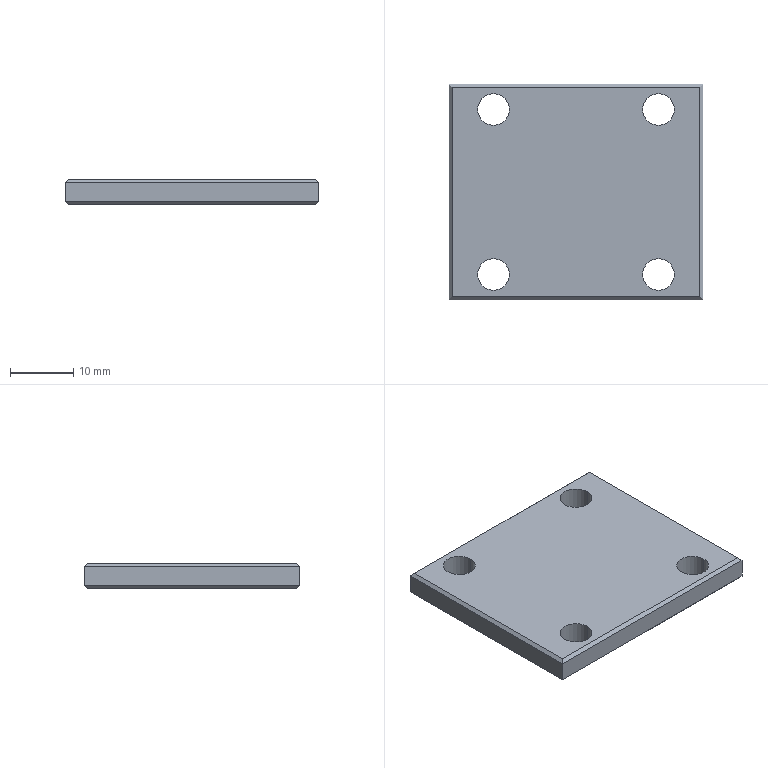Part | NX | 1 solid | 30 faces | box 40 x 34 x 4.05 mm | volume 5145 mm3 | plane 14 | cylinder 8 | cone 8 | commonest cylinder face diameters 5 x8
STEP:
#1=CARTESIAN_POINT('',(0.5,-0.5,3.45));
#2=VERTEX_POINT('',#1);
#3=CARTESIAN_POINT('',(0.5,-33.5,3.45));
#4=VERTEX_POINT('',#3);
#5=CARTESIAN_POINT('',(0.5,0.,3.45));
#6=DIRECTION('',(0.,-1.,0.));
#7=VECTOR('',#6,1000.);
#8=LINE('',#5,#7);
#9=EDGE_CURVE('',#2,#4,#8,.T.);
#10=ORIENTED_EDGE('',*,*,#9,.T.);
#11=CARTESIAN_POINT('',(39.5,-33.5,3.45));
#12=VERTEX_POINT('',#11);
#13=CARTESIAN_POINT('',(0.,-33.5,3.45));
#14=DIRECTION('',(1.,0.,0.));
#15=VECTOR('',#14,1000.);
#16=LINE('',#13,#15);
#17=EDGE_CURVE('',#4,#12,#16,.T.);
#18=ORIENTED_EDGE('',*,*,#17,.T.);
#19=CARTESIAN_POINT('',(39.5,-0.5,3.45));
#20=VERTEX_POINT('',#19);
#21=CARTESIAN_POINT('',(39.5,0.,3.45));
#22=DIRECTION('',(0.,1.,0.));
#23=VECTOR('',#22,1000.);
#24=LINE('',#21,#23);
#25=EDGE_CURVE('',#12,#20,#24,.T.);
#26=ORIENTED_EDGE('',*,*,#25,.T.);
#27=CARTESIAN_POINT('',(0.,-0.5,3.45));
#28=DIRECTION('',(-1.,0.,0.));
#29=VECTOR('',#28,1000.);
#30=LINE('',#27,#29);
#31=EDGE_CURVE('',#20,#2,#30,.T.);
#32=ORIENTED_EDGE('',*,*,#31,.T.);
#33=EDGE_LOOP('',(#10,#18,#26,#32));
#34=FACE_BOUND('',#33,.T.);
#35=CARTESIAN_POINT('',(30.5,-4.,3.45));
#36=VERTEX_POINT('',#35);
#37=CARTESIAN_POINT('',(35.5,-4.,3.45));
#38=VERTEX_POINT('',#37);
#39=CARTESIAN_POINT('',(33.,-4.,3.45));
#40=DIRECTION('',(0.,0.,-1.));
#41=DIRECTION('',(-1.,0.,0.));
#42=AXIS2_PLACEMENT_3D('',#39,#40,#41);
#43=CIRCLE('',#42,2.5);
#44=EDGE_CURVE('',#36,#38,#43,.T.);
#45=ORIENTED_EDGE('',*,*,#44,.T.);
#46=CARTESIAN_POINT('',(33.,-4.,3.45));
#47=DIRECTION('',(0.,0.,-1.));
#48=DIRECTION('',(-1.,0.,0.));
#49=AXIS2_PLACEMENT_3D('',#46,#47,#48);
#50=CIRCLE('',#49,2.5);
#51=EDGE_CURVE('',#38,#36,#50,.T.);
#52=ORIENTED_EDGE('',*,*,#51,.T.);
#53=EDGE_LOOP('',(#45,#52));
#54=FACE_BOUND('',#53,.T.);
#55=CARTESIAN_POINT('',(35.5,-30.,3.45));
#56=VERTEX_POINT('',#55);
#57=CARTESIAN_POINT('',(30.5,-30.,3.45));
#58=VERTEX_POINT('',#57);
#59=CARTESIAN_POINT('',(33.,-30.,3.45));
#60=DIRECTION('',(0.,0.,-1.));
#61=DIRECTION('',(-1.,0.,0.));
#62=AXIS2_PLACEMENT_3D('',#59,#60,#61);
#63=CIRCLE('',#62,2.5);
#64=EDGE_CURVE('',#56,#58,#63,.T.);
#65=ORIENTED_EDGE('',*,*,#64,.T.);
#66=CARTESIAN_POINT('',(33.,-30.,3.45));
#67=DIRECTION('',(0.,0.,-1.));
#68=DIRECTION('',(-1.,0.,0.));
#69=AXIS2_PLACEMENT_3D('',#66,#67,#68);
#70=CIRCLE('',#69,2.5);
#71=EDGE_CURVE('',#58,#56,#70,.T.);
#72=ORIENTED_EDGE('',*,*,#71,.T.);
#73=EDGE_LOOP('',(#65,#72));
#74=FACE_BOUND('',#73,.T.);
#75=CARTESIAN_POINT('',(4.5,-4.,3.45));
#76=VERTEX_POINT('',#75);
#77=CARTESIAN_POINT('',(9.5,-4.,3.45));
#78=VERTEX_POINT('',#77);
#79=CARTESIAN_POINT('',(7.,-4.,3.45));
#80=DIRECTION('',(0.,0.,-1.));
#81=DIRECTION('',(-1.,0.,0.));
#82=AXIS2_PLACEMENT_3D('',#79,#80,#81);
#83=CIRCLE('',#82,2.5);
#84=EDGE_CURVE('',#76,#78,#83,.T.);
#85=ORIENTED_EDGE('',*,*,#84,.T.);
#86=CARTESIAN_POINT('',(7.,-4.,3.45));
#87=DIRECTION('',(0.,0.,-1.));
#88=DIRECTION('',(-1.,0.,0.));
#89=AXIS2_PLACEMENT_3D('',#86,#87,#88);
#90=CIRCLE('',#89,2.5);
#91=EDGE_CURVE('',#78,#76,#90,.T.);
#92=ORIENTED_EDGE('',*,*,#91,.T.);
#93=EDGE_LOOP('',(#85,#92));
#94=FACE_BOUND('',#93,.T.);
#95=CARTESIAN_POINT('',(4.5,-30.,3.45));
#96=VERTEX_POINT('',#95);
#97=CARTESIAN_POINT('',(9.5,-30.,3.45));
#98=VERTEX_POINT('',#97);
#99=CARTESIAN_POINT('',(7.,-30.,3.45));
#100=DIRECTION('',(0.,0.,-1.));
#101=DIRECTION('',(-1.,0.,0.));
#102=AXIS2_PLACEMENT_3D('',#99,#100,#101);
#103=CIRCLE('',#102,2.5);
#104=EDGE_CURVE('',#96,#98,#103,.T.);
#105=ORIENTED_EDGE('',*,*,#104,.T.);
#106=CARTESIAN_POINT('',(7.,-30.,3.45));
#107=DIRECTION('',(0.,0.,-1.));
#108=DIRECTION('',(-1.,0.,0.));
#109=AXIS2_PLACEMENT_3D('',#106,#107,#108);
#110=CIRCLE('',#109,2.5);
#111=EDGE_CURVE('',#98,#96,#110,.T.);
#112=ORIENTED_EDGE('',*,*,#111,.T.);
#113=EDGE_LOOP('',(#105,#112));
#114=FACE_BOUND('',#113,.T.);
#115=CARTESIAN_POINT('',(40.,62.,3.45));
#116=DIRECTION('',(0.,0.,-1.));
#117=DIRECTION('',(0.,-1.,0.));
#118=AXIS2_PLACEMENT_3D('',#115,#116,#117);
#119=PLANE('',#118);
#120=ADVANCED_FACE('',(#34,#54,#74,#94,#114),#119,.F.);
#121=CARTESIAN_POINT('',(0.,-34.,2.95));
#122=VERTEX_POINT('',#121);
#123=CARTESIAN_POINT('',(40.,-34.,2.95));
#124=VERTEX_POINT('',#123);
#125=CARTESIAN_POINT('',(0.,-34.,2.95));
#126=DIRECTION('',(1.,0.,0.));
#127=VECTOR('',#126,1000.);
#128=LINE('',#125,#127);
#129=EDGE_CURVE('',#122,#124,#128,.T.);
#130=ORIENTED_EDGE('',*,*,#129,.F.);
#131=CARTESIAN_POINT('',(0.,-34.,-0.1));
#132=VERTEX_POINT('',#131);
#133=CARTESIAN_POINT('',(0.,-34.,0.));
#134=DIRECTION('',(0.,0.,-1.));
#135=VECTOR('',#134,1000.);
#136=LINE('',#133,#135);
#137=EDGE_CURVE('',#122,#132,#136,.T.);
#138=ORIENTED_EDGE('',*,*,#137,.T.);
#139=CARTESIAN_POINT('',(40.,-34.,-0.1));
#140=VERTEX_POINT('',#139);
#141=CARTESIAN_POINT('',(0.,-34.,-0.1));
#142=DIRECTION('',(-1.,0.,0.));
#143=VECTOR('',#142,1000.);
#144=LINE('',#141,#143);
#145=EDGE_CURVE('',#140,#132,#144,.T.);
#146=ORIENTED_EDGE('',*,*,#145,.F.);
#147=CARTESIAN_POINT('',(40.,-34.,0.));
#148=DIRECTION('',(0.,0.,1.));
#149=VECTOR('',#148,1000.);
#150=LINE('',#147,#149);
#151=EDGE_CURVE('',#140,#124,#150,.T.);
#152=ORIENTED_EDGE('',*,*,#151,.T.);
#153=EDGE_LOOP('',(#130,#138,#146,#152));
#154=FACE_BOUND('',#153,.T.);
#155=CARTESIAN_POINT('',(0.,-34.,0.));
#156=DIRECTION('',(0.,-1.,0.));
#157=DIRECTION('',(0.,0.,-1.));
#158=AXIS2_PLACEMENT_3D('',#155,#156,#157);
#159=PLANE('',#158);
#160=ADVANCED_FACE('',(#154),#159,.T.);
#161=ORIENTED_EDGE('',*,*,#44,.F.);
#162=CARTESIAN_POINT('',(30.5,-4.,-0.1));
#163=VERTEX_POINT('',#162);
#164=CARTESIAN_POINT('',(30.5,-4.,10.5));
#165=DIRECTION('',(0.,0.,-1.));
#166=VECTOR('',#165,1000.);
#167=LINE('',#164,#166);
#168=EDGE_CURVE('',#163,#36,#167,.F.);
#169=ORIENTED_EDGE('',*,*,#168,.F.);
#170=CARTESIAN_POINT('',(35.5,-4.,-0.1));
#171=VERTEX_POINT('',#170);
#172=CARTESIAN_POINT('',(33.,-4.,-0.1));
#173=DIRECTION('',(0.,0.,-1.));
#174=DIRECTION('',(-1.,0.,0.));
#175=AXIS2_PLACEMENT_3D('',#172,#173,#174);
#176=CIRCLE('',#175,2.5);
#177=EDGE_CURVE('',#163,#171,#176,.T.);
#178=ORIENTED_EDGE('',*,*,#177,.T.);
#179=CARTESIAN_POINT('',(35.5,-4.,10.5));
#180=DIRECTION('',(0.,0.,-1.));
#181=VECTOR('',#180,1000.);
#182=LINE('',#179,#181);
#183=EDGE_CURVE('',#171,#38,#182,.F.);
#184=ORIENTED_EDGE('',*,*,#183,.T.);
#185=EDGE_LOOP('',(#161,#169,#178,#184));
#186=FACE_BOUND('',#185,.T.);
#187=CARTESIAN_POINT('',(33.,-4.,10.5));
#188=DIRECTION('',(0.,0.,-1.));
#189=DIRECTION('',(-1.,0.,0.));
#190=AXIS2_PLACEMENT_3D('',#187,#188,#189);
#191=CYLINDRICAL_SURFACE('',#190,2.5);
#192=ADVANCED_FACE('',(#186),#191,.F.);
#193=ORIENTED_EDGE('',*,*,#104,.F.);
#194=CARTESIAN_POINT('',(4.5,-30.,-0.1));
#195=VERTEX_POINT('',#194);
#196=CARTESIAN_POINT('',(4.5,-30.,10.5));
#197=DIRECTION('',(0.,0.,-1.));
#198=VECTOR('',#197,1000.);
#199=LINE('',#196,#198);
#200=EDGE_CURVE('',#195,#96,#199,.F.);
#201=ORIENTED_EDGE('',*,*,#200,.F.);
#202=CARTESIAN_POINT('',(9.5,-30.,-0.1));
#203=VERTEX_POINT('',#202);
#204=CARTESIAN_POINT('',(7.,-30.,-0.1));
#205=DIRECTION('',(0.,0.,-1.));
#206=DIRECTION('',(-1.,0.,0.));
#207=AXIS2_PLACEMENT_3D('',#204,#205,#206);
#208=CIRCLE('',#207,2.5);
#209=EDGE_CURVE('',#195,#203,#208,.T.);
#210=ORIENTED_EDGE('',*,*,#209,.T.);
#211=CARTESIAN_POINT('',(9.5,-30.,10.5));
#212=DIRECTION('',(0.,0.,-1.));
#213=VECTOR('',#212,1000.);
#214=LINE('',#211,#213);
#215=EDGE_CURVE('',#203,#98,#214,.F.);
#216=ORIENTED_EDGE('',*,*,#215,.T.);
#217=EDGE_LOOP('',(#193,#201,#210,#216));
#218=FACE_BOUND('',#217,.T.);
#219=CARTESIAN_POINT('',(7.,-30.,10.5));
#220=DIRECTION('',(0.,0.,-1.));
#221=DIRECTION('',(-1.,0.,0.));
#222=AXIS2_PLACEMENT_3D('',#219,#220,#221);
#223=CYLINDRICAL_SURFACE('',#222,2.5);
#224=ADVANCED_FACE('',(#218),#223,.F.);
#225=CARTESIAN_POINT('',(9.5,-4.,-0.1));
#226=VERTEX_POINT('',#225);
#227=CARTESIAN_POINT('',(4.5,-4.,-0.1));
#228=VERTEX_POINT('',#227);
#229=CARTESIAN_POINT('',(7.,-4.,-0.1));
#230=DIRECTION('',(0.,0.,-1.));
#231=DIRECTION('',(-1.,0.,0.));
#232=AXIS2_PLACEMENT_3D('',#229,#230,#231);
#233=CIRCLE('',#232,2.5);
#234=EDGE_CURVE('',#226,#228,#233,.T.);
#235=ORIENTED_EDGE('',*,*,#234,.T.);
#236=CARTESIAN_POINT('',(4.5,-4.,10.5));
#237=DIRECTION('',(0.,0.,-1.));
#238=VECTOR('',#237,1000.);
#239=LINE('',#236,#238);
#240=EDGE_CURVE('',#228,#76,#239,.F.);
#241=ORIENTED_EDGE('',*,*,#240,.T.);
#242=ORIENTED_EDGE('',*,*,#91,.F.);
#243=CARTESIAN_POINT('',(9.5,-4.,10.5));
#244=DIRECTION('',(0.,0.,-1.));
#245=VECTOR('',#244,1000.);
#246=LINE('',#243,#245);
#247=EDGE_CURVE('',#226,#78,#246,.F.);
#248=ORIENTED_EDGE('',*,*,#247,.F.);
#249=EDGE_LOOP('',(#235,#241,#242,#248));
#250=FACE_BOUND('',#249,.T.);
#251=CARTESIAN_POINT('',(7.,-4.,10.5));
#252=DIRECTION('',(0.,0.,-1.));
#253=DIRECTION('',(-1.,0.,0.));
#254=AXIS2_PLACEMENT_3D('',#251,#252,#253);
#255=CYLINDRICAL_SURFACE('',#254,2.5);
#256=ADVANCED_FACE('',(#250),#255,.F.);
#257=CARTESIAN_POINT('',(0.,0.,2.95));
#258=VERTEX_POINT('',#257);
#259=CARTESIAN_POINT('',(0.,0.,2.95));
#260=DIRECTION('',(0.,-1.,0.));
#261=VECTOR('',#260,1000.);
#262=LINE('',#259,#261);
#263=EDGE_CURVE('',#258,#122,#262,.T.);
#264=ORIENTED_EDGE('',*,*,#263,.F.);
#265=CARTESIAN_POINT('',(0.,0.,-0.1));
#266=VERTEX_POINT('',#265);
#267=CARTESIAN_POINT('',(0.,0.,0.));
#268=DIRECTION('',(0.,0.,1.));
#269=VECTOR('',#268,1000.);
#270=LINE('',#267,#269);
#271=EDGE_CURVE('',#266,#258,#270,.T.);
#272=ORIENTED_EDGE('',*,*,#271,.F.);
#273=CARTESIAN_POINT('',(0.,0.,-0.1));
#274=DIRECTION('',(0.,-1.,0.));
#275=VECTOR('',#274,1000.);
#276=LINE('',#273,#275);
#277=EDGE_CURVE('',#266,#132,#276,.T.);
#278=ORIENTED_EDGE('',*,*,#277,.T.);
#279=ORIENTED_EDGE('',*,*,#137,.F.);
#280=EDGE_LOOP('',(#264,#272,#278,#279));
#281=FACE_BOUND('',#280,.T.);
#282=CARTESIAN_POINT('',(0.,0.,0.));
#283=DIRECTION('',(-1.,0.,0.));
#284=DIRECTION('',(0.,0.,1.));
#285=AXIS2_PLACEMENT_3D('',#282,#283,#284);
#286=PLANE('',#285);
#287=ADVANCED_FACE('',(#281),#286,.T.);
#288=ORIENTED_EDGE('',*,*,#64,.F.);
#289=CARTESIAN_POINT('',(35.5,-30.,-0.1));
#290=VERTEX_POINT('',#289);
#291=CARTESIAN_POINT('',(35.5,-30.,10.5));
#292=DIRECTION('',(0.,0.,-1.));
#293=VECTOR('',#292,1000.);
#294=LINE('',#291,#293);
#295=EDGE_CURVE('',#290,#56,#294,.F.);
#296=ORIENTED_EDGE('',*,*,#295,.F.);
#297=CARTESIAN_POINT('',(30.5,-30.,-0.1));
#298=VERTEX_POINT('',#297);
#299=CARTESIAN_POINT('',(33.,-30.,-0.1));
#300=DIRECTION('',(0.,0.,-1.));
#301=DIRECTION('',(-1.,0.,0.));
#302=AXIS2_PLACEMENT_3D('',#299,#300,#301);
#303=CIRCLE('',#302,2.5);
#304=EDGE_CURVE('',#290,#298,#303,.T.);
#305=ORIENTED_EDGE('',*,*,#304,.T.);
#306=CARTESIAN_POINT('',(30.5,-30.,10.5));
#307=DIRECTION('',(0.,0.,-1.));
#308=VECTOR('',#307,1000.);
#309=LINE('',#306,#308);
#310=EDGE_CURVE('',#298,#58,#309,.F.);
#311=ORIENTED_EDGE('',*,*,#310,.T.);
#312=EDGE_LOOP('',(#288,#296,#305,#311));
#313=FACE_BOUND('',#312,.T.);
#314=CARTESIAN_POINT('',(33.,-30.,10.5));
#315=DIRECTION('',(0.,0.,-1.));
#316=DIRECTION('',(-1.,0.,0.));
#317=AXIS2_PLACEMENT_3D('',#314,#315,#316);
#318=CYLINDRICAL_SURFACE('',#317,2.5);
#319=ADVANCED_FACE('',(#313),#318,.F.);
#320=CARTESIAN_POINT('',(33.,-4.,-0.1));
#321=DIRECTION('',(0.,0.,-1.));
#322=DIRECTION('',(-1.,0.,0.));
#323=AXIS2_PLACEMENT_3D('',#320,#321,#322);
#324=CIRCLE('',#323,2.5);
#325=EDGE_CURVE('',#171,#163,#324,.T.);
#326=ORIENTED_EDGE('',*,*,#325,.F.);
#327=CARTESIAN_POINT('',(36.,-4.,-0.6));
#328=VERTEX_POINT('',#327);
#329=CARTESIAN_POINT('',(36.,-4.,-0.6));
#330=DIRECTION('',(0.7071,0.,-0.7071));
#331=VECTOR('',#330,1000.);
#332=LINE('',#329,#331);
#333=EDGE_CURVE('',#171,#328,#332,.T.);
#334=ORIENTED_EDGE('',*,*,#333,.T.);
#335=CARTESIAN_POINT('',(30.,-4.,-0.6));
#336=VERTEX_POINT('',#335);
#337=CARTESIAN_POINT('',(33.,-4.,-0.6));
#338=DIRECTION('',(0.,0.,-1.));
#339=DIRECTION('',(-1.,0.,0.));
#340=AXIS2_PLACEMENT_3D('',#337,#338,#339);
#341=CIRCLE('',#340,3.);
#342=EDGE_CURVE('',#328,#336,#341,.T.);
#343=ORIENTED_EDGE('',*,*,#342,.T.);
#344=CARTESIAN_POINT('',(30.,-4.,-0.6));
#345=DIRECTION('',(-0.7071,0.,-0.7071));
#346=VECTOR('',#345,1000.);
#347=LINE('',#344,#346);
#348=EDGE_CURVE('',#163,#336,#347,.T.);
#349=ORIENTED_EDGE('',*,*,#348,.F.);
#350=EDGE_LOOP('',(#326,#334,#343,#349));
#351=FACE_BOUND('',#350,.T.);
#352=CARTESIAN_POINT('',(33.,-4.,-0.6));
#353=DIRECTION('',(0.,0.,-1.));
#354=DIRECTION('',(-1.,0.,0.));
#355=AXIS2_PLACEMENT_3D('',#352,#353,#354);
#356=CONICAL_SURFACE('',#355,3.,0.7854);
#357=ADVANCED_FACE('',(#351),#356,.F.);
#358=CARTESIAN_POINT('',(40.,0.,2.95));
#359=VERTEX_POINT('',#358);
#360=CARTESIAN_POINT('',(0.,0.,2.95));
#361=DIRECTION('',(-1.,0.,0.));
#362=VECTOR('',#361,1000.);
#363=LINE('',#360,#362);
#364=EDGE_CURVE('',#359,#258,#363,.T.);
#365=ORIENTED_EDGE('',*,*,#364,.F.);
#366=CARTESIAN_POINT('',(40.,0.,-0.1));
#367=VERTEX_POINT('',#366);
#368=CARTESIAN_POINT('',(40.,0.,0.));
#369=DIRECTION('',(0.,0.,-1.));
#370=VECTOR('',#369,1000.);
#371=LINE('',#368,#370);
#372=EDGE_CURVE('',#359,#367,#371,.T.);
#373=ORIENTED_EDGE('',*,*,#372,.T.);
#374=CARTESIAN_POINT('',(0.,0.,-0.1));
#375=DIRECTION('',(1.,0.,0.));
#376=VECTOR('',#375,1000.);
#377=LINE('',#374,#376);
#378=EDGE_CURVE('',#266,#367,#377,.T.);
#379=ORIENTED_EDGE('',*,*,#378,.F.);
#380=ORIENTED_EDGE('',*,*,#271,.T.);
#381=EDGE_LOOP('',(#365,#373,#379,#380));
#382=FACE_BOUND('',#381,.T.);
#383=CARTESIAN_POINT('',(40.,0.,0.));
#384=DIRECTION('',(0.,1.,0.));
#385=DIRECTION('',(1.,0.,0.));
#386=AXIS2_PLACEMENT_3D('',#383,#384,#385);
#387=PLANE('',#386);
#388=ADVANCED_FACE('',(#382),#387,.T.);
#389=CARTESIAN_POINT('',(40.,0.,2.95));
#390=DIRECTION('',(0.,1.,0.));
#391=VECTOR('',#390,1000.);
#392=LINE('',#389,#391);
#393=EDGE_CURVE('',#124,#359,#392,.T.);
#394=ORIENTED_EDGE('',*,*,#393,.F.);
#395=ORIENTED_EDGE('',*,*,#151,.F.);
#396=CARTESIAN_POINT('',(40.,0.,-0.1));
#397=DIRECTION('',(0.,1.,0.));
#398=VECTOR('',#397,1000.);
#399=LINE('',#396,#398);
#400=EDGE_CURVE('',#140,#367,#399,.T.);
#401=ORIENTED_EDGE('',*,*,#400,.T.);
#402=ORIENTED_EDGE('',*,*,#372,.F.);
#403=EDGE_LOOP('',(#394,#395,#401,#402));
#404=FACE_BOUND('',#403,.T.);
#405=CARTESIAN_POINT('',(40.,-34.,0.));
#406=DIRECTION('',(1.,0.,0.));
#407=DIRECTION('',(0.,1.,0.));
#408=AXIS2_PLACEMENT_3D('',#405,#406,#407);
#409=PLANE('',#408);
#410=ADVANCED_FACE('',(#404),#409,.T.);
#411=CARTESIAN_POINT('',(39.5,-0.5,-0.6));
#412=VERTEX_POINT('',#411);
#413=CARTESIAN_POINT('',(39.5,-33.5,-0.6));
#414=VERTEX_POINT('',#413);
#415=CARTESIAN_POINT('',(39.5,0.,-0.6));
#416=DIRECTION('',(0.,-1.,0.));
#417=VECTOR('',#416,1000.);
#418=LINE('',#415,#417);
#419=EDGE_CURVE('',#412,#414,#418,.T.);
#420=ORIENTED_EDGE('',*,*,#419,.F.);
#421=CARTESIAN_POINT('',(40.1,0.1,0.));
#422=DIRECTION('',(0.5774,0.5774,0.5774));
#423=VECTOR('',#422,1000.);
#424=LINE('',#421,#423);
#425=EDGE_CURVE('',#412,#367,#424,.T.);
#426=ORIENTED_EDGE('',*,*,#425,.T.);
#427=ORIENTED_EDGE('',*,*,#400,.F.);
#428=CARTESIAN_POINT('',(40.1,-34.1,0.));
#429=DIRECTION('',(-0.5774,0.5774,-0.5774));
#430=VECTOR('',#429,1000.);
#431=LINE('',#428,#430);
#432=EDGE_CURVE('',#140,#414,#431,.T.);
#433=ORIENTED_EDGE('',*,*,#432,.T.);
#434=EDGE_LOOP('',(#420,#426,#427,#433));
#435=FACE_BOUND('',#434,.T.);
#436=CARTESIAN_POINT('',(39.75,-17.,-0.35));
#437=DIRECTION('',(-0.7071,0.,0.7071));
#438=DIRECTION('',(0.,1.,0.));
#439=AXIS2_PLACEMENT_3D('',#436,#437,#438);
#440=PLANE('',#439);
#441=ADVANCED_FACE('',(#435),#440,.F.);
#442=CARTESIAN_POINT('',(0.5,-33.5,-0.6));
#443=VERTEX_POINT('',#442);
#444=CARTESIAN_POINT('',(0.,-33.5,-0.6));
#445=DIRECTION('',(-1.,0.,0.));
#446=VECTOR('',#445,1000.);
#447=LINE('',#444,#446);
#448=EDGE_CURVE('',#414,#443,#447,.T.);
#449=ORIENTED_EDGE('',*,*,#448,.F.);
#450=ORIENTED_EDGE('',*,*,#432,.F.);
#451=ORIENTED_EDGE('',*,*,#145,.T.);
#452=CARTESIAN_POINT('',(-0.1,-34.1,0.));
#453=DIRECTION('',(-0.5774,-0.5774,0.5774));
#454=VECTOR('',#453,1000.);
#455=LINE('',#452,#454);
#456=EDGE_CURVE('',#443,#132,#455,.T.);
#457=ORIENTED_EDGE('',*,*,#456,.F.);
#458=EDGE_LOOP('',(#449,#450,#451,#457));
#459=FACE_BOUND('',#458,.T.);
#460=CARTESIAN_POINT('',(20.,-33.75,-0.35));
#461=DIRECTION('',(0.,0.7071,0.7071));
#462=DIRECTION('',(1.,0.,0.));
#463=AXIS2_PLACEMENT_3D('',#460,#461,#462);
#464=PLANE('',#463);
#465=ADVANCED_FACE('',(#459),#464,.F.);
#466=CARTESIAN_POINT('',(0.5,-0.5,-0.6));
#467=VERTEX_POINT('',#466);
#468=CARTESIAN_POINT('',(0.5,0.,-0.6));
#469=DIRECTION('',(0.,1.,0.));
#470=VECTOR('',#469,1000.);
#471=LINE('',#468,#470);
#472=EDGE_CURVE('',#443,#467,#471,.T.);
#473=ORIENTED_EDGE('',*,*,#472,.F.);
#474=ORIENTED_EDGE('',*,*,#456,.T.);
#475=ORIENTED_EDGE('',*,*,#277,.F.);
#476=CARTESIAN_POINT('',(-0.1,0.1,0.));
#477=DIRECTION('',(0.5774,-0.5774,-0.5774));
#478=VECTOR('',#477,1000.);
#479=LINE('',#476,#478);
#480=EDGE_CURVE('',#266,#467,#479,.T.);
#481=ORIENTED_EDGE('',*,*,#480,.T.);
#482=EDGE_LOOP('',(#473,#474,#475,#481));
#483=FACE_BOUND('',#482,.T.);
#484=CARTESIAN_POINT('',(0.25,-17.,-0.35));
#485=DIRECTION('',(0.7071,0.,0.7071));
#486=DIRECTION('',(0.,-1.,0.));
#487=AXIS2_PLACEMENT_3D('',#484,#485,#486);
#488=PLANE('',#487);
#489=ADVANCED_FACE('',(#483),#488,.F.);
#490=CARTESIAN_POINT('',(0.,-0.5,-0.6));
#491=DIRECTION('',(1.,0.,0.));
#492=VECTOR('',#491,1000.);
#493=LINE('',#490,#492);
#494=EDGE_CURVE('',#467,#412,#493,.T.);
#495=ORIENTED_EDGE('',*,*,#494,.F.);
#496=ORIENTED_EDGE('',*,*,#480,.F.);
#497=ORIENTED_EDGE('',*,*,#378,.T.);
#498=ORIENTED_EDGE('',*,*,#425,.F.);
#499=EDGE_LOOP('',(#495,#496,#497,#498));
#500=FACE_BOUND('',#499,.T.);
#501=CARTESIAN_POINT('',(20.,-0.25,-0.35));
#502=DIRECTION('',(0.,-0.7071,0.7071));
#503=DIRECTION('',(-1.,0.,0.));
#504=AXIS2_PLACEMENT_3D('',#501,#502,#503);
#505=PLANE('',#504);
#506=ADVANCED_FACE('',(#500),#505,.F.);
#507=CARTESIAN_POINT('',(4.,-30.,-0.6));
#508=VERTEX_POINT('',#507);
#509=CARTESIAN_POINT('',(10.,-30.,-0.6));
#510=VERTEX_POINT('',#509);
#511=CARTESIAN_POINT('',(7.,-30.,-0.6));
#512=DIRECTION('',(0.,0.,-1.));
#513=DIRECTION('',(-1.,0.,0.));
#514=AXIS2_PLACEMENT_3D('',#511,#512,#513);
#515=CIRCLE('',#514,3.);
#516=EDGE_CURVE('',#508,#510,#515,.T.);
#517=ORIENTED_EDGE('',*,*,#516,.T.);
#518=CARTESIAN_POINT('',(10.,-30.,-0.6));
#519=DIRECTION('',(0.7071,0.,-0.7071));
#520=VECTOR('',#519,1000.);
#521=LINE('',#518,#520);
#522=EDGE_CURVE('',#203,#510,#521,.T.);
#523=ORIENTED_EDGE('',*,*,#522,.F.);
#524=ORIENTED_EDGE('',*,*,#209,.F.);
#525=CARTESIAN_POINT('',(4.,-30.,-0.6));
#526=DIRECTION('',(-0.7071,0.,-0.7071));
#527=VECTOR('',#526,1000.);
#528=LINE('',#525,#527);
#529=EDGE_CURVE('',#195,#508,#528,.T.);
#530=ORIENTED_EDGE('',*,*,#529,.T.);
#531=EDGE_LOOP('',(#517,#523,#524,#530));
#532=FACE_BOUND('',#531,.T.);
#533=CARTESIAN_POINT('',(7.,-30.,-0.6));
#534=DIRECTION('',(0.,0.,-1.));
#535=DIRECTION('',(-1.,0.,0.));
#536=AXIS2_PLACEMENT_3D('',#533,#534,#535);
#537=CONICAL_SURFACE('',#536,3.,0.7854);
#538=ADVANCED_FACE('',(#532),#537,.F.);
#539=CARTESIAN_POINT('',(4.,-4.,-0.6));
#540=VERTEX_POINT('',#539);
#541=CARTESIAN_POINT('',(10.,-4.,-0.6));
#542=VERTEX_POINT('',#541);
#543=CARTESIAN_POINT('',(7.,-4.,-0.6));
#544=DIRECTION('',(0.,0.,-1.));
#545=DIRECTION('',(-1.,0.,0.));
#546=AXIS2_PLACEMENT_3D('',#543,#544,#545);
#547=CIRCLE('',#546,3.);
#548=EDGE_CURVE('',#540,#542,#547,.T.);
#549=ORIENTED_EDGE('',*,*,#548,.T.);
#550=CARTESIAN_POINT('',(10.,-4.,-0.6));
#551=DIRECTION('',(0.7071,0.,-0.7071));
#552=VECTOR('',#551,1000.);
#553=LINE('',#550,#552);
#554=EDGE_CURVE('',#226,#542,#553,.T.);
#555=ORIENTED_EDGE('',*,*,#554,.F.);
#556=CARTESIAN_POINT('',(7.,-4.,-0.1));
#557=DIRECTION('',(0.,0.,-1.));
#558=DIRECTION('',(-1.,0.,0.));
#559=AXIS2_PLACEMENT_3D('',#556,#557,#558);
#560=CIRCLE('',#559,2.5);
#561=EDGE_CURVE('',#228,#226,#560,.T.);
#562=ORIENTED_EDGE('',*,*,#561,.F.);
#563=CARTESIAN_POINT('',(4.,-4.,-0.6));
#564=DIRECTION('',(-0.7071,0.,-0.7071));
#565=VECTOR('',#564,1000.);
#566=LINE('',#563,#565);
#567=EDGE_CURVE('',#228,#540,#566,.T.);
#568=ORIENTED_EDGE('',*,*,#567,.T.);
#569=EDGE_LOOP('',(#549,#555,#562,#568));
#570=FACE_BOUND('',#569,.T.);
#571=CARTESIAN_POINT('',(7.,-4.,-0.6));
#572=DIRECTION('',(0.,0.,-1.));
#573=DIRECTION('',(-1.,0.,0.));
#574=AXIS2_PLACEMENT_3D('',#571,#572,#573);
#575=CONICAL_SURFACE('',#574,3.,0.7854);
#576=ADVANCED_FACE('',(#570),#575,.F.);
#577=CARTESIAN_POINT('',(30.,-30.,-0.6));
#578=VERTEX_POINT('',#577);
#579=CARTESIAN_POINT('',(36.,-30.,-0.6));
#580=VERTEX_POINT('',#579);
#581=CARTESIAN_POINT('',(33.,-30.,-0.6));
#582=DIRECTION('',(0.,0.,-1.));
#583=DIRECTION('',(-1.,0.,0.));
#584=AXIS2_PLACEMENT_3D('',#581,#582,#583);
#585=CIRCLE('',#584,3.);
#586=EDGE_CURVE('',#578,#580,#585,.T.);
#587=ORIENTED_EDGE('',*,*,#586,.T.);
#588=CARTESIAN_POINT('',(36.,-30.,-0.6));
#589=DIRECTION('',(0.7071,0.,-0.7071));
#590=VECTOR('',#589,1000.);
#591=LINE('',#588,#590);
#592=EDGE_CURVE('',#290,#580,#591,.T.);
#593=ORIENTED_EDGE('',*,*,#592,.F.);
#594=CARTESIAN_POINT('',(33.,-30.,-0.1));
#595=DIRECTION('',(0.,0.,-1.));
#596=DIRECTION('',(-1.,0.,0.));
#597=AXIS2_PLACEMENT_3D('',#594,#595,#596);
#598=CIRCLE('',#597,2.5);
#599=EDGE_CURVE('',#298,#290,#598,.T.);
#600=ORIENTED_EDGE('',*,*,#599,.F.);
#601=CARTESIAN_POINT('',(30.,-30.,-0.6));
#602=DIRECTION('',(-0.7071,0.,-0.7071));
#603=VECTOR('',#602,1000.);
#604=LINE('',#601,#603);
#605=EDGE_CURVE('',#298,#578,#604,.T.);
#606=ORIENTED_EDGE('',*,*,#605,.T.);
#607=EDGE_LOOP('',(#587,#593,#600,#606));
#608=FACE_BOUND('',#607,.T.);
#609=CARTESIAN_POINT('',(33.,-30.,-0.6));
#610=DIRECTION('',(0.,0.,-1.));
#611=DIRECTION('',(-1.,0.,0.));
#612=AXIS2_PLACEMENT_3D('',#609,#610,#611);
#613=CONICAL_SURFACE('',#612,3.,0.7854);
#614=ADVANCED_FACE('',(#608),#613,.F.);
#615=ORIENTED_EDGE('',*,*,#494,.T.);
#616=ORIENTED_EDGE('',*,*,#419,.T.);
#617=ORIENTED_EDGE('',*,*,#448,.T.);
#618=ORIENTED_EDGE('',*,*,#472,.T.);
#619=EDGE_LOOP('',(#615,#616,#617,#618));
#620=FACE_BOUND('',#619,.T.);
#621=ORIENTED_EDGE('',*,*,#548,.F.);
#622=CARTESIAN_POINT('',(7.,-4.,-0.6));
#623=DIRECTION('',(0.,0.,-1.));
#624=DIRECTION('',(-1.,0.,0.));
#625=AXIS2_PLACEMENT_3D('',#622,#623,#624);
#626=CIRCLE('',#625,3.);
#627=EDGE_CURVE('',#542,#540,#626,.T.);
#628=ORIENTED_EDGE('',*,*,#627,.F.);
#629=EDGE_LOOP('',(#621,#628));
#630=FACE_BOUND('',#629,.T.);
#631=ORIENTED_EDGE('',*,*,#586,.F.);
#632=CARTESIAN_POINT('',(33.,-30.,-0.6));
#633=DIRECTION('',(0.,0.,-1.));
#634=DIRECTION('',(-1.,0.,0.));
#635=AXIS2_PLACEMENT_3D('',#632,#633,#634);
#636=CIRCLE('',#635,3.);
#637=EDGE_CURVE('',#580,#578,#636,.T.);
#638=ORIENTED_EDGE('',*,*,#637,.F.);
#639=EDGE_LOOP('',(#631,#638));
#640=FACE_BOUND('',#639,.T.);
#641=CARTESIAN_POINT('',(33.,-4.,-0.6));
#642=DIRECTION('',(0.,0.,-1.));
#643=DIRECTION('',(-1.,0.,0.));
#644=AXIS2_PLACEMENT_3D('',#641,#642,#643);
#645=CIRCLE('',#644,3.);
#646=EDGE_CURVE('',#336,#328,#645,.T.);
#647=ORIENTED_EDGE('',*,*,#646,.F.);
#648=ORIENTED_EDGE('',*,*,#342,.F.);
#649=EDGE_LOOP('',(#647,#648));
#650=FACE_BOUND('',#649,.T.);
#651=ORIENTED_EDGE('',*,*,#516,.F.);
#652=CARTESIAN_POINT('',(7.,-30.,-0.6));
#653=DIRECTION('',(0.,0.,-1.));
#654=DIRECTION('',(-1.,0.,0.));
#655=AXIS2_PLACEMENT_3D('',#652,#653,#654);
#656=CIRCLE('',#655,3.);
#657=EDGE_CURVE('',#510,#508,#656,.T.);
#658=ORIENTED_EDGE('',*,*,#657,.F.);
#659=EDGE_LOOP('',(#651,#658));
#660=FACE_BOUND('',#659,.T.);
#661=CARTESIAN_POINT('',(0.,0.,-0.6));
#662=DIRECTION('',(0.,0.,1.));
#663=DIRECTION('',(1.,0.,0.));
#664=AXIS2_PLACEMENT_3D('',#661,#662,#663);
#665=PLANE('',#664);
#666=ADVANCED_FACE('',(#620,#630,#640,#650,#660),#665,.F.);
#667=ORIENTED_EDGE('',*,*,#263,.T.);
#668=CARTESIAN_POINT('',(-2.95,-36.95,0.));
#669=DIRECTION('',(0.5774,0.5774,0.5774));
#670=VECTOR('',#669,1000.);
#671=LINE('',#668,#670);
#672=EDGE_CURVE('',#122,#4,#671,.T.);
#673=ORIENTED_EDGE('',*,*,#672,.T.);
#674=ORIENTED_EDGE('',*,*,#9,.F.);
#675=CARTESIAN_POINT('',(-2.95,2.95,0.));
#676=DIRECTION('',(0.5774,-0.5774,0.5774));
#677=VECTOR('',#676,1000.);
#678=LINE('',#675,#677);
#679=EDGE_CURVE('',#258,#2,#678,.T.);
#680=ORIENTED_EDGE('',*,*,#679,.F.);
#681=EDGE_LOOP('',(#667,#673,#674,#680));
#682=FACE_BOUND('',#681,.T.);
#683=CARTESIAN_POINT('',(0.25,-17.,3.2));
#684=DIRECTION('',(-0.7071,0.,0.7071));
#685=DIRECTION('',(0.,1.,0.));
#686=AXIS2_PLACEMENT_3D('',#683,#684,#685);
#687=PLANE('',#686);
#688=ADVANCED_FACE('',(#682),#687,.T.);
#689=ORIENTED_EDGE('',*,*,#129,.T.);
#690=CARTESIAN_POINT('',(42.95,-36.95,0.));
#691=DIRECTION('',(0.5774,-0.5774,-0.5774));
#692=VECTOR('',#691,1000.);
#693=LINE('',#690,#692);
#694=EDGE_CURVE('',#12,#124,#693,.T.);
#695=ORIENTED_EDGE('',*,*,#694,.F.);
#696=ORIENTED_EDGE('',*,*,#17,.F.);
#697=ORIENTED_EDGE('',*,*,#672,.F.);
#698=EDGE_LOOP('',(#689,#695,#696,#697));
#699=FACE_BOUND('',#698,.T.);
#700=CARTESIAN_POINT('',(20.,-33.75,3.2));
#701=DIRECTION('',(0.,-0.7071,0.7071));
#702=DIRECTION('',(-1.,0.,0.));
#703=AXIS2_PLACEMENT_3D('',#700,#701,#702);
#704=PLANE('',#703);
#705=ADVANCED_FACE('',(#699),#704,.T.);
#706=ORIENTED_EDGE('',*,*,#364,.T.);
#707=ORIENTED_EDGE('',*,*,#679,.T.);
#708=ORIENTED_EDGE('',*,*,#31,.F.);
#709=CARTESIAN_POINT('',(42.95,2.95,0.));
#710=DIRECTION('',(0.5774,0.5774,-0.5774));
#711=VECTOR('',#710,1000.);
#712=LINE('',#709,#711);
#713=EDGE_CURVE('',#20,#359,#712,.T.);
#714=ORIENTED_EDGE('',*,*,#713,.T.);
#715=EDGE_LOOP('',(#706,#707,#708,#714));
#716=FACE_BOUND('',#715,.T.);
#717=CARTESIAN_POINT('',(20.,-0.25,3.2));
#718=DIRECTION('',(0.,0.7071,0.7071));
#719=DIRECTION('',(1.,0.,0.));
#720=AXIS2_PLACEMENT_3D('',#717,#718,#719);
#721=PLANE('',#720);
#722=ADVANCED_FACE('',(#716),#721,.T.);
#723=ORIENTED_EDGE('',*,*,#393,.T.);
#724=ORIENTED_EDGE('',*,*,#713,.F.);
#725=ORIENTED_EDGE('',*,*,#25,.F.);
#726=ORIENTED_EDGE('',*,*,#694,.T.);
#727=EDGE_LOOP('',(#723,#724,#725,#726));
#728=FACE_BOUND('',#727,.T.);
#729=CARTESIAN_POINT('',(39.75,-17.,3.2));
#730=DIRECTION('',(0.7071,0.,0.7071));
#731=DIRECTION('',(0.,-1.,0.));
#732=AXIS2_PLACEMENT_3D('',#729,#730,#731);
#733=PLANE('',#732);
#734=ADVANCED_FACE('',(#728),#733,.T.);
#735=ORIENTED_EDGE('',*,*,#84,.F.);
#736=ORIENTED_EDGE('',*,*,#240,.F.);
#737=ORIENTED_EDGE('',*,*,#561,.T.);
#738=ORIENTED_EDGE('',*,*,#247,.T.);
#739=EDGE_LOOP('',(#735,#736,#737,#738));
#740=FACE_BOUND('',#739,.T.);
#741=CARTESIAN_POINT('',(7.,-4.,10.5));
#742=DIRECTION('',(0.,0.,-1.));
#743=DIRECTION('',(-1.,0.,0.));
#744=AXIS2_PLACEMENT_3D('',#741,#742,#743);
#745=CYLINDRICAL_SURFACE('',#744,2.5);
#746=ADVANCED_FACE('',(#740),#745,.F.);
#747=ORIENTED_EDGE('',*,*,#234,.F.);
#748=ORIENTED_EDGE('',*,*,#554,.T.);
#749=ORIENTED_EDGE('',*,*,#627,.T.);
#750=ORIENTED_EDGE('',*,*,#567,.F.);
#751=EDGE_LOOP('',(#747,#748,#749,#750));
#752=FACE_BOUND('',#751,.T.);
#753=CARTESIAN_POINT('',(7.,-4.,-0.6));
#754=DIRECTION('',(0.,0.,-1.));
#755=DIRECTION('',(-1.,0.,0.));
#756=AXIS2_PLACEMENT_3D('',#753,#754,#755);
#757=CONICAL_SURFACE('',#756,3.,0.7854);
#758=ADVANCED_FACE('',(#752),#757,.F.);
#759=CARTESIAN_POINT('',(7.,-30.,-0.1));
#760=DIRECTION('',(0.,0.,-1.));
#761=DIRECTION('',(-1.,0.,0.));
#762=AXIS2_PLACEMENT_3D('',#759,#760,#761);
#763=CIRCLE('',#762,2.5);
#764=EDGE_CURVE('',#203,#195,#763,.T.);
#765=ORIENTED_EDGE('',*,*,#764,.T.);
#766=ORIENTED_EDGE('',*,*,#200,.T.);
#767=ORIENTED_EDGE('',*,*,#111,.F.);
#768=ORIENTED_EDGE('',*,*,#215,.F.);
#769=EDGE_LOOP('',(#765,#766,#767,#768));
#770=FACE_BOUND('',#769,.T.);
#771=CARTESIAN_POINT('',(7.,-30.,10.5));
#772=DIRECTION('',(0.,0.,-1.));
#773=DIRECTION('',(-1.,0.,0.));
#774=AXIS2_PLACEMENT_3D('',#771,#772,#773);
#775=CYLINDRICAL_SURFACE('',#774,2.5);
#776=ADVANCED_FACE('',(#770),#775,.F.);
#777=ORIENTED_EDGE('',*,*,#764,.F.);
#778=ORIENTED_EDGE('',*,*,#522,.T.);
#779=ORIENTED_EDGE('',*,*,#657,.T.);
#780=ORIENTED_EDGE('',*,*,#529,.F.);
#781=EDGE_LOOP('',(#777,#778,#779,#780));
#782=FACE_BOUND('',#781,.T.);
#783=CARTESIAN_POINT('',(7.,-30.,-0.6));
#784=DIRECTION('',(0.,0.,-1.));
#785=DIRECTION('',(-1.,0.,0.));
#786=AXIS2_PLACEMENT_3D('',#783,#784,#785);
#787=CONICAL_SURFACE('',#786,3.,0.7854);
#788=ADVANCED_FACE('',(#782),#787,.F.);
#789=ORIENTED_EDGE('',*,*,#325,.T.);
#790=ORIENTED_EDGE('',*,*,#168,.T.);
#791=ORIENTED_EDGE('',*,*,#51,.F.);
#792=ORIENTED_EDGE('',*,*,#183,.F.);
#793=EDGE_LOOP('',(#789,#790,#791,#792));
#794=FACE_BOUND('',#793,.T.);
#795=CARTESIAN_POINT('',(33.,-4.,10.5));
#796=DIRECTION('',(0.,0.,-1.));
#797=DIRECTION('',(-1.,0.,0.));
#798=AXIS2_PLACEMENT_3D('',#795,#796,#797);
#799=CYLINDRICAL_SURFACE('',#798,2.5);
#800=ADVANCED_FACE('',(#794),#799,.F.);
#801=ORIENTED_EDGE('',*,*,#646,.T.);
#802=ORIENTED_EDGE('',*,*,#333,.F.);
#803=ORIENTED_EDGE('',*,*,#177,.F.);
#804=ORIENTED_EDGE('',*,*,#348,.T.);
#805=EDGE_LOOP('',(#801,#802,#803,#804));
#806=FACE_BOUND('',#805,.T.);
#807=CARTESIAN_POINT('',(33.,-4.,-0.6));
#808=DIRECTION('',(0.,0.,-1.));
#809=DIRECTION('',(-1.,0.,0.));
#810=AXIS2_PLACEMENT_3D('',#807,#808,#809);
#811=CONICAL_SURFACE('',#810,3.,0.7854);
#812=ADVANCED_FACE('',(#806),#811,.F.);
#813=ORIENTED_EDGE('',*,*,#310,.F.);
#814=ORIENTED_EDGE('',*,*,#599,.T.);
#815=ORIENTED_EDGE('',*,*,#295,.T.);
#816=ORIENTED_EDGE('',*,*,#71,.F.);
#817=EDGE_LOOP('',(#813,#814,#815,#816));
#818=FACE_BOUND('',#817,.T.);
#819=CARTESIAN_POINT('',(33.,-30.,10.5));
#820=DIRECTION('',(0.,0.,-1.));
#821=DIRECTION('',(-1.,0.,0.));
#822=AXIS2_PLACEMENT_3D('',#819,#820,#821);
#823=CYLINDRICAL_SURFACE('',#822,2.5);
#824=ADVANCED_FACE('',(#818),#823,.F.);
#825=ORIENTED_EDGE('',*,*,#304,.F.);
#826=ORIENTED_EDGE('',*,*,#592,.T.);
#827=ORIENTED_EDGE('',*,*,#637,.T.);
#828=ORIENTED_EDGE('',*,*,#605,.F.);
#829=EDGE_LOOP('',(#825,#826,#827,#828));
#830=FACE_BOUND('',#829,.T.);
#831=CARTESIAN_POINT('',(33.,-30.,-0.6));
#832=DIRECTION('',(0.,0.,-1.));
#833=DIRECTION('',(-1.,0.,0.));
#834=AXIS2_PLACEMENT_3D('',#831,#832,#833);
#835=CONICAL_SURFACE('',#834,3.,0.7854);
#836=ADVANCED_FACE('',(#830),#835,.F.);
#837=CLOSED_SHELL('',(#120,#160,#192,#224,#256,#287,#319,#357,#388,#410,#441,#465,#489,#506,#538,#576,#614,#666,#688,#705,#722,#734,#746,#758,#776,#788,#800,#812,#824,#836));
#838=MANIFOLD_SOLID_BREP('',#837);
#839=(LENGTH_UNIT()NAMED_UNIT(*)SI_UNIT(.MILLI.,.METRE.));
#840=UNCERTAINTY_MEASURE_WITH_UNIT(LENGTH_MEASURE(0.00001),#839,'','');
#841=(NAMED_UNIT(*)PLANE_ANGLE_UNIT()SI_UNIT($,.RADIAN.));
#842=(NAMED_UNIT(*)SI_UNIT($,.STERADIAN.)SOLID_ANGLE_UNIT());
#843=(GEOMETRIC_REPRESENTATION_CONTEXT(3)GLOBAL_UNCERTAINTY_ASSIGNED_CONTEXT((#840))GLOBAL_UNIT_ASSIGNED_CONTEXT((#839,#841,#842))REPRESENTATION_CONTEXT('',''));
#844=ADVANCED_BREP_SHAPE_REPRESENTATION('',(#838),#843);